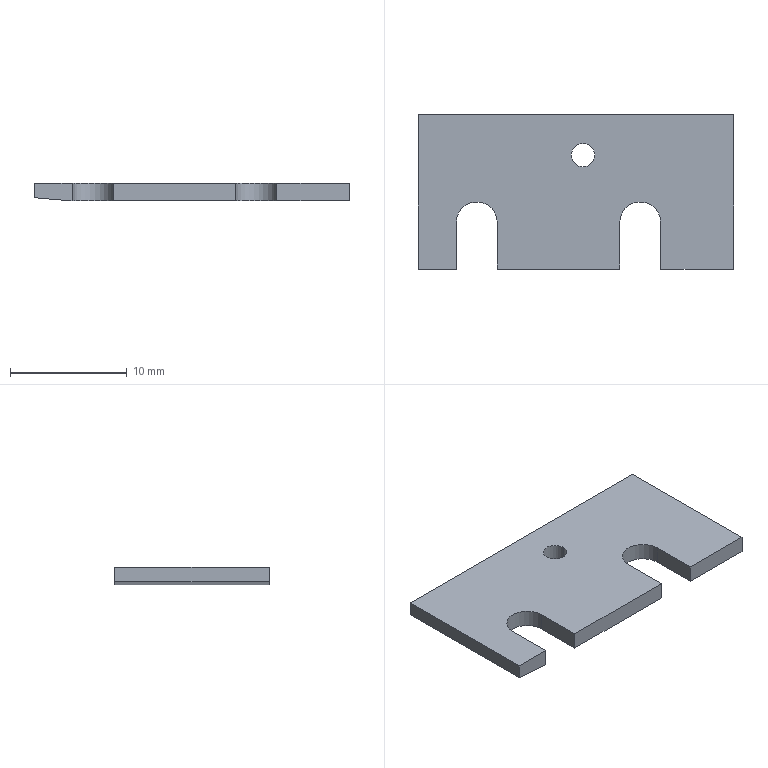Part | NX | 1 solid | 17 faces | box 27 x 13.2 x 1.5 mm | volume 468.259 mm3 | plane 13 | cylinder 4 | commonest cylinder face diameters 2 x2 3.5 x2
STEP:
#1=CARTESIAN_POINT('',(-113.5,7.2,-0.75));
#2=VERTEX_POINT('',#1);
#3=CARTESIAN_POINT('',(-113.5,-6.,-0.75));
#4=VERTEX_POINT('',#3);
#5=CARTESIAN_POINT('',(-113.5,0.,-0.75));
#6=DIRECTION('',(0.,-1.,0.));
#7=VECTOR('',#6,1000.);
#8=LINE('',#5,#7);
#9=EDGE_CURVE('',#2,#4,#8,.T.);
#10=ORIENTED_EDGE('',*,*,#9,.T.);
#11=CARTESIAN_POINT('',(-119.75,-6.,-0.75));
#12=VERTEX_POINT('',#11);
#13=CARTESIAN_POINT('',(0.,-6.,-0.75));
#14=DIRECTION('',(-1.,0.,0.));
#15=VECTOR('',#14,1000.);
#16=LINE('',#13,#15);
#17=EDGE_CURVE('',#4,#12,#16,.T.);
#18=ORIENTED_EDGE('',*,*,#17,.T.);
#19=CARTESIAN_POINT('',(-119.75,-2.,-0.75));
#20=VERTEX_POINT('',#19);
#21=CARTESIAN_POINT('',(-119.75,0.,-0.75));
#22=DIRECTION('',(0.,1.,0.));
#23=VECTOR('',#22,1000.);
#24=LINE('',#21,#23);
#25=EDGE_CURVE('',#12,#20,#24,.T.);
#26=ORIENTED_EDGE('',*,*,#25,.T.);
#27=CARTESIAN_POINT('',(-123.25,-2.,-0.75));
#28=VERTEX_POINT('',#27);
#29=CARTESIAN_POINT('',(-121.5,-2.,-0.75));
#30=DIRECTION('',(0.,0.,1.));
#31=DIRECTION('',(1.,0.,0.));
#32=AXIS2_PLACEMENT_3D('',#29,#30,#31);
#33=CIRCLE('',#32,1.75);
#34=EDGE_CURVE('',#20,#28,#33,.T.);
#35=ORIENTED_EDGE('',*,*,#34,.T.);
#36=CARTESIAN_POINT('',(-123.25,-6.,-0.75));
#37=VERTEX_POINT('',#36);
#38=CARTESIAN_POINT('',(-123.25,0.,-0.75));
#39=DIRECTION('',(0.,-1.,0.));
#40=VECTOR('',#39,1000.);
#41=LINE('',#38,#40);
#42=EDGE_CURVE('',#28,#37,#41,.T.);
#43=ORIENTED_EDGE('',*,*,#42,.T.);
#44=CARTESIAN_POINT('',(-133.75,-6.,-0.75));
#45=VERTEX_POINT('',#44);
#46=CARTESIAN_POINT('',(0.,-6.,-0.75));
#47=DIRECTION('',(-1.,0.,0.));
#48=VECTOR('',#47,1000.);
#49=LINE('',#46,#48);
#50=EDGE_CURVE('',#37,#45,#49,.T.);
#51=ORIENTED_EDGE('',*,*,#50,.T.);
#52=CARTESIAN_POINT('',(-133.75,-2.,-0.75));
#53=VERTEX_POINT('',#52);
#54=CARTESIAN_POINT('',(-133.75,0.,-0.75));
#55=DIRECTION('',(0.,1.,0.));
#56=VECTOR('',#55,1000.);
#57=LINE('',#54,#56);
#58=EDGE_CURVE('',#45,#53,#57,.T.);
#59=ORIENTED_EDGE('',*,*,#58,.T.);
#60=CARTESIAN_POINT('',(-137.25,-2.,-0.75));
#61=VERTEX_POINT('',#60);
#62=CARTESIAN_POINT('',(-135.5,-2.,-0.75));
#63=DIRECTION('',(0.,0.,1.));
#64=DIRECTION('',(1.,0.,0.));
#65=AXIS2_PLACEMENT_3D('',#62,#63,#64);
#66=CIRCLE('',#65,1.75);
#67=EDGE_CURVE('',#53,#61,#66,.T.);
#68=ORIENTED_EDGE('',*,*,#67,.T.);
#69=CARTESIAN_POINT('',(-137.25,-6.,-0.75));
#70=VERTEX_POINT('',#69);
#71=CARTESIAN_POINT('',(-137.25,0.,-0.75));
#72=DIRECTION('',(0.,-1.,0.));
#73=VECTOR('',#72,1000.);
#74=LINE('',#71,#73);
#75=EDGE_CURVE('',#61,#70,#74,.T.);
#76=ORIENTED_EDGE('',*,*,#75,.T.);
#77=CARTESIAN_POINT('',(-137.5,-6.,-0.75));
#78=VERTEX_POINT('',#77);
#79=CARTESIAN_POINT('',(0.,-6.,-0.75));
#80=DIRECTION('',(-1.,0.,0.));
#81=VECTOR('',#80,1000.);
#82=LINE('',#79,#81);
#83=EDGE_CURVE('',#70,#78,#82,.T.);
#84=ORIENTED_EDGE('',*,*,#83,.T.);
#85=CARTESIAN_POINT('',(-137.5,7.2,-0.75));
#86=VERTEX_POINT('',#85);
#87=CARTESIAN_POINT('',(-137.5,0.,-0.75));
#88=DIRECTION('',(0.,1.,0.));
#89=VECTOR('',#88,1000.);
#90=LINE('',#87,#89);
#91=EDGE_CURVE('',#78,#86,#90,.T.);
#92=ORIENTED_EDGE('',*,*,#91,.T.);
#93=CARTESIAN_POINT('',(0.,7.2,-0.75));
#94=DIRECTION('',(-1.,0.,0.));
#95=VECTOR('',#94,1000.);
#96=LINE('',#93,#95);
#97=EDGE_CURVE('',#2,#86,#96,.T.);
#98=ORIENTED_EDGE('',*,*,#97,.F.);
#99=EDGE_LOOP('',(#10,#18,#26,#35,#43,#51,#59,#68,#76,#84,#92,#98));
#100=FACE_BOUND('',#99,.T.);
#101=CARTESIAN_POINT('',(-127.4,3.75,-0.75));
#102=VERTEX_POINT('',#101);
#103=CARTESIAN_POINT('',(-125.4,3.75,-0.75));
#104=VERTEX_POINT('',#103);
#105=CARTESIAN_POINT('',(-126.4,3.75,-0.75));
#106=DIRECTION('',(0.,0.,-1.));
#107=DIRECTION('',(-1.,0.,0.));
#108=AXIS2_PLACEMENT_3D('',#105,#106,#107);
#109=CIRCLE('',#108,1.);
#110=EDGE_CURVE('',#102,#104,#109,.T.);
#111=ORIENTED_EDGE('',*,*,#110,.F.);
#112=CARTESIAN_POINT('',(-126.4,3.75,-0.75));
#113=DIRECTION('',(0.,0.,-1.));
#114=DIRECTION('',(-1.,0.,0.));
#115=AXIS2_PLACEMENT_3D('',#112,#113,#114);
#116=CIRCLE('',#115,1.);
#117=EDGE_CURVE('',#104,#102,#116,.T.);
#118=ORIENTED_EDGE('',*,*,#117,.F.);
#119=EDGE_LOOP('',(#111,#118));
#120=FACE_BOUND('',#119,.T.);
#121=CARTESIAN_POINT('',(-127.,0.,-0.75));
#122=DIRECTION('',(0.,0.,-1.));
#123=DIRECTION('',(0.,-1.,0.));
#124=AXIS2_PLACEMENT_3D('',#121,#122,#123);
#125=PLANE('',#124);
#126=ADVANCED_FACE('',(#100,#120),#125,.T.);
#127=ORIENTED_EDGE('',*,*,#9,.F.);
#128=CARTESIAN_POINT('',(-113.5,7.2,0.75));
#129=VERTEX_POINT('',#128);
#130=CARTESIAN_POINT('',(-113.5,7.2,0.));
#131=DIRECTION('',(0.,0.,1.));
#132=VECTOR('',#131,1000.);
#133=LINE('',#130,#132);
#134=EDGE_CURVE('',#2,#129,#133,.T.);
#135=ORIENTED_EDGE('',*,*,#134,.T.);
#136=CARTESIAN_POINT('',(-113.5,-6.,0.75));
#137=VERTEX_POINT('',#136);
#138=CARTESIAN_POINT('',(-113.5,0.,0.75));
#139=DIRECTION('',(0.,1.,0.));
#140=VECTOR('',#139,1000.);
#141=LINE('',#138,#140);
#142=EDGE_CURVE('',#137,#129,#141,.T.);
#143=ORIENTED_EDGE('',*,*,#142,.F.);
#144=CARTESIAN_POINT('',(-113.5,-6.,0.));
#145=DIRECTION('',(0.,0.,1.));
#146=VECTOR('',#145,1000.);
#147=LINE('',#144,#146);
#148=EDGE_CURVE('',#4,#137,#147,.T.);
#149=ORIENTED_EDGE('',*,*,#148,.F.);
#150=EDGE_LOOP('',(#127,#135,#143,#149));
#151=FACE_BOUND('',#150,.T.);
#152=CARTESIAN_POINT('',(-113.5,6.,-0.75));
#153=DIRECTION('',(-1.,0.,0.));
#154=DIRECTION('',(0.,0.,1.));
#155=AXIS2_PLACEMENT_3D('',#152,#153,#154);
#156=PLANE('',#155);
#157=ADVANCED_FACE('',(#151),#156,.F.);
#158=ORIENTED_EDGE('',*,*,#83,.F.);
#159=CARTESIAN_POINT('',(-137.25,-6.,0.75));
#160=VERTEX_POINT('',#159);
#161=CARTESIAN_POINT('',(-137.25,-6.,-0.9));
#162=DIRECTION('',(0.,0.,1.));
#163=VECTOR('',#162,1000.);
#164=LINE('',#161,#163);
#165=EDGE_CURVE('',#70,#160,#164,.T.);
#166=ORIENTED_EDGE('',*,*,#165,.T.);
#167=CARTESIAN_POINT('',(-140.5,-6.,0.75));
#168=VERTEX_POINT('',#167);
#169=CARTESIAN_POINT('',(0.,-6.,0.75));
#170=DIRECTION('',(-1.,0.,0.));
#171=VECTOR('',#170,1000.);
#172=LINE('',#169,#171);
#173=EDGE_CURVE('',#160,#168,#172,.T.);
#174=ORIENTED_EDGE('',*,*,#173,.T.);
#175=CARTESIAN_POINT('',(-140.5,-6.,-0.4875));
#176=VERTEX_POINT('',#175);
#177=CARTESIAN_POINT('',(-140.5,-6.,0.));
#178=DIRECTION('',(0.,0.,-1.));
#179=VECTOR('',#178,1000.);
#180=LINE('',#177,#179);
#181=EDGE_CURVE('',#168,#176,#180,.T.);
#182=ORIENTED_EDGE('',*,*,#181,.T.);
#183=CARTESIAN_POINT('',(0.,-6.,-12.78));
#184=DIRECTION('',(0.9962,0.,-0.08716));
#185=VECTOR('',#184,1000.);
#186=LINE('',#183,#185);
#187=EDGE_CURVE('',#176,#78,#186,.T.);
#188=ORIENTED_EDGE('',*,*,#187,.T.);
#189=EDGE_LOOP('',(#158,#166,#174,#182,#188));
#190=FACE_BOUND('',#189,.T.);
#191=CARTESIAN_POINT('',(-113.5,-6.,-0.75));
#192=DIRECTION('',(0.,1.,0.));
#193=DIRECTION('',(1.,0.,0.));
#194=AXIS2_PLACEMENT_3D('',#191,#192,#193);
#195=PLANE('',#194);
#196=ADVANCED_FACE('',(#190),#195,.F.);
#197=ORIENTED_EDGE('',*,*,#91,.F.);
#198=ORIENTED_EDGE('',*,*,#187,.F.);
#199=CARTESIAN_POINT('',(-140.5,7.2,-0.4875));
#200=VERTEX_POINT('',#199);
#201=CARTESIAN_POINT('',(-140.5,0.,-0.4875));
#202=DIRECTION('',(0.,1.,0.));
#203=VECTOR('',#202,1000.);
#204=LINE('',#201,#203);
#205=EDGE_CURVE('',#176,#200,#204,.T.);
#206=ORIENTED_EDGE('',*,*,#205,.T.);
#207=CARTESIAN_POINT('',(0.,7.2,-12.78));
#208=DIRECTION('',(0.9962,0.,-0.08716));
#209=VECTOR('',#208,1000.);
#210=LINE('',#207,#209);
#211=EDGE_CURVE('',#200,#86,#210,.T.);
#212=ORIENTED_EDGE('',*,*,#211,.T.);
#213=EDGE_LOOP('',(#197,#198,#206,#212));
#214=FACE_BOUND('',#213,.T.);
#215=CARTESIAN_POINT('',(-137.5,-6.,-0.75));
#216=DIRECTION('',(0.08716,0.,0.9962));
#217=DIRECTION('',(0.,-1.,0.));
#218=AXIS2_PLACEMENT_3D('',#215,#216,#217);
#219=PLANE('',#218);
#220=ADVANCED_FACE('',(#214),#219,.F.);
#221=ORIENTED_EDGE('',*,*,#97,.T.);
#222=ORIENTED_EDGE('',*,*,#211,.F.);
#223=CARTESIAN_POINT('',(-140.5,7.2,0.75));
#224=VERTEX_POINT('',#223);
#225=CARTESIAN_POINT('',(-140.5,7.2,0.));
#226=DIRECTION('',(0.,0.,-1.));
#227=VECTOR('',#226,1000.);
#228=LINE('',#225,#227);
#229=EDGE_CURVE('',#224,#200,#228,.T.);
#230=ORIENTED_EDGE('',*,*,#229,.F.);
#231=CARTESIAN_POINT('',(0.,7.2,0.75));
#232=DIRECTION('',(-1.,0.,0.));
#233=VECTOR('',#232,1000.);
#234=LINE('',#231,#233);
#235=EDGE_CURVE('',#129,#224,#234,.T.);
#236=ORIENTED_EDGE('',*,*,#235,.F.);
#237=ORIENTED_EDGE('',*,*,#134,.F.);
#238=EDGE_LOOP('',(#221,#222,#230,#236,#237));
#239=FACE_BOUND('',#238,.T.);
#240=CARTESIAN_POINT('',(-140.5,7.2,-0.75));
#241=DIRECTION('',(0.,-1.,0.));
#242=DIRECTION('',(0.,0.,-1.));
#243=AXIS2_PLACEMENT_3D('',#240,#241,#242);
#244=PLANE('',#243);
#245=ADVANCED_FACE('',(#239),#244,.F.);
#246=ORIENTED_EDGE('',*,*,#142,.T.);
#247=ORIENTED_EDGE('',*,*,#235,.T.);
#248=CARTESIAN_POINT('',(-140.5,0.,0.75));
#249=DIRECTION('',(0.,-1.,0.));
#250=VECTOR('',#249,1000.);
#251=LINE('',#248,#250);
#252=EDGE_CURVE('',#224,#168,#251,.T.);
#253=ORIENTED_EDGE('',*,*,#252,.T.);
#254=ORIENTED_EDGE('',*,*,#173,.F.);
#255=CARTESIAN_POINT('',(-137.25,-2.,0.75));
#256=VERTEX_POINT('',#255);
#257=CARTESIAN_POINT('',(-137.25,0.,0.75));
#258=DIRECTION('',(0.,-1.,0.));
#259=VECTOR('',#258,1000.);
#260=LINE('',#257,#259);
#261=EDGE_CURVE('',#256,#160,#260,.T.);
#262=ORIENTED_EDGE('',*,*,#261,.F.);
#263=CARTESIAN_POINT('',(-133.75,-2.,0.75));
#264=VERTEX_POINT('',#263);
#265=CARTESIAN_POINT('',(-135.5,-2.,0.75));
#266=DIRECTION('',(0.,0.,1.));
#267=DIRECTION('',(1.,0.,0.));
#268=AXIS2_PLACEMENT_3D('',#265,#266,#267);
#269=CIRCLE('',#268,1.75);
#270=EDGE_CURVE('',#264,#256,#269,.T.);
#271=ORIENTED_EDGE('',*,*,#270,.F.);
#272=CARTESIAN_POINT('',(-133.75,-6.,0.75));
#273=VERTEX_POINT('',#272);
#274=CARTESIAN_POINT('',(-133.75,0.,0.75));
#275=DIRECTION('',(0.,1.,0.));
#276=VECTOR('',#275,1000.);
#277=LINE('',#274,#276);
#278=EDGE_CURVE('',#273,#264,#277,.T.);
#279=ORIENTED_EDGE('',*,*,#278,.F.);
#280=CARTESIAN_POINT('',(-123.25,-6.,0.75));
#281=VERTEX_POINT('',#280);
#282=CARTESIAN_POINT('',(0.,-6.,0.75));
#283=DIRECTION('',(-1.,0.,0.));
#284=VECTOR('',#283,1000.);
#285=LINE('',#282,#284);
#286=EDGE_CURVE('',#281,#273,#285,.T.);
#287=ORIENTED_EDGE('',*,*,#286,.F.);
#288=CARTESIAN_POINT('',(-123.25,-2.,0.75));
#289=VERTEX_POINT('',#288);
#290=CARTESIAN_POINT('',(-123.25,0.,0.75));
#291=DIRECTION('',(0.,-1.,0.));
#292=VECTOR('',#291,1000.);
#293=LINE('',#290,#292);
#294=EDGE_CURVE('',#289,#281,#293,.T.);
#295=ORIENTED_EDGE('',*,*,#294,.F.);
#296=CARTESIAN_POINT('',(-119.75,-2.,0.75));
#297=VERTEX_POINT('',#296);
#298=CARTESIAN_POINT('',(-121.5,-2.,0.75));
#299=DIRECTION('',(0.,0.,1.));
#300=DIRECTION('',(1.,0.,0.));
#301=AXIS2_PLACEMENT_3D('',#298,#299,#300);
#302=CIRCLE('',#301,1.75);
#303=EDGE_CURVE('',#297,#289,#302,.T.);
#304=ORIENTED_EDGE('',*,*,#303,.F.);
#305=CARTESIAN_POINT('',(-119.75,-6.,0.75));
#306=VERTEX_POINT('',#305);
#307=CARTESIAN_POINT('',(-119.75,0.,0.75));
#308=DIRECTION('',(0.,1.,0.));
#309=VECTOR('',#308,1000.);
#310=LINE('',#307,#309);
#311=EDGE_CURVE('',#306,#297,#310,.T.);
#312=ORIENTED_EDGE('',*,*,#311,.F.);
#313=CARTESIAN_POINT('',(0.,-6.,0.75));
#314=DIRECTION('',(-1.,0.,0.));
#315=VECTOR('',#314,1000.);
#316=LINE('',#313,#315);
#317=EDGE_CURVE('',#137,#306,#316,.T.);
#318=ORIENTED_EDGE('',*,*,#317,.F.);
#319=EDGE_LOOP('',(#246,#247,#253,#254,#262,#271,#279,#287,#295,#304,#312,#318));
#320=FACE_BOUND('',#319,.T.);
#321=CARTESIAN_POINT('',(-127.4,3.75,0.75));
#322=VERTEX_POINT('',#321);
#323=CARTESIAN_POINT('',(-125.4,3.75,0.75));
#324=VERTEX_POINT('',#323);
#325=CARTESIAN_POINT('',(-126.4,3.75,0.75));
#326=DIRECTION('',(0.,0.,-1.));
#327=DIRECTION('',(-1.,0.,0.));
#328=AXIS2_PLACEMENT_3D('',#325,#326,#327);
#329=CIRCLE('',#328,1.);
#330=EDGE_CURVE('',#322,#324,#329,.T.);
#331=ORIENTED_EDGE('',*,*,#330,.T.);
#332=CARTESIAN_POINT('',(-126.4,3.75,0.75));
#333=DIRECTION('',(0.,0.,-1.));
#334=DIRECTION('',(-1.,0.,0.));
#335=AXIS2_PLACEMENT_3D('',#332,#333,#334);
#336=CIRCLE('',#335,1.);
#337=EDGE_CURVE('',#324,#322,#336,.T.);
#338=ORIENTED_EDGE('',*,*,#337,.T.);
#339=EDGE_LOOP('',(#331,#338));
#340=FACE_BOUND('',#339,.T.);
#341=CARTESIAN_POINT('',(-127.,0.,0.75));
#342=DIRECTION('',(0.,0.,-1.));
#343=DIRECTION('',(0.,-1.,0.));
#344=AXIS2_PLACEMENT_3D('',#341,#342,#343);
#345=PLANE('',#344);
#346=ADVANCED_FACE('',(#320,#340),#345,.F.);
#347=ORIENTED_EDGE('',*,*,#205,.F.);
#348=ORIENTED_EDGE('',*,*,#181,.F.);
#349=ORIENTED_EDGE('',*,*,#252,.F.);
#350=ORIENTED_EDGE('',*,*,#229,.T.);
#351=EDGE_LOOP('',(#347,#348,#349,#350));
#352=FACE_BOUND('',#351,.T.);
#353=CARTESIAN_POINT('',(-140.5,-6.,-0.75));
#354=DIRECTION('',(1.,0.,0.));
#355=DIRECTION('',(0.,1.,0.));
#356=AXIS2_PLACEMENT_3D('',#353,#354,#355);
#357=PLANE('',#356);
#358=ADVANCED_FACE('',(#352),#357,.F.);
#359=ORIENTED_EDGE('',*,*,#303,.T.);
#360=CARTESIAN_POINT('',(-123.25,-2.,0.75));
#361=DIRECTION('',(0.,0.,1.));
#362=VECTOR('',#361,1000.);
#363=LINE('',#360,#362);
#364=EDGE_CURVE('',#28,#289,#363,.T.);
#365=ORIENTED_EDGE('',*,*,#364,.F.);
#366=ORIENTED_EDGE('',*,*,#34,.F.);
#367=CARTESIAN_POINT('',(-119.75,-2.,0.75));
#368=DIRECTION('',(0.,0.,1.));
#369=VECTOR('',#368,1000.);
#370=LINE('',#367,#369);
#371=EDGE_CURVE('',#20,#297,#370,.T.);
#372=ORIENTED_EDGE('',*,*,#371,.T.);
#373=EDGE_LOOP('',(#359,#365,#366,#372));
#374=FACE_BOUND('',#373,.T.);
#375=CARTESIAN_POINT('',(-121.5,-2.,0.75));
#376=DIRECTION('',(0.,0.,1.));
#377=DIRECTION('',(1.,0.,0.));
#378=AXIS2_PLACEMENT_3D('',#375,#376,#377);
#379=CYLINDRICAL_SURFACE('',#378,1.75);
#380=ADVANCED_FACE('',(#374),#379,.F.);
#381=ORIENTED_EDGE('',*,*,#330,.F.);
#382=CARTESIAN_POINT('',(-127.4,3.75,0.75));
#383=DIRECTION('',(0.,0.,-1.));
#384=VECTOR('',#383,1000.);
#385=LINE('',#382,#384);
#386=EDGE_CURVE('',#102,#322,#385,.F.);
#387=ORIENTED_EDGE('',*,*,#386,.F.);
#388=ORIENTED_EDGE('',*,*,#110,.T.);
#389=CARTESIAN_POINT('',(-125.4,3.75,0.75));
#390=DIRECTION('',(0.,0.,-1.));
#391=VECTOR('',#390,1000.);
#392=LINE('',#389,#391);
#393=EDGE_CURVE('',#104,#324,#392,.F.);
#394=ORIENTED_EDGE('',*,*,#393,.T.);
#395=EDGE_LOOP('',(#381,#387,#388,#394));
#396=FACE_BOUND('',#395,.T.);
#397=CARTESIAN_POINT('',(-126.4,3.75,0.75));
#398=DIRECTION('',(0.,0.,-1.));
#399=DIRECTION('',(-1.,0.,0.));
#400=AXIS2_PLACEMENT_3D('',#397,#398,#399);
#401=CYLINDRICAL_SURFACE('',#400,1.);
#402=ADVANCED_FACE('',(#396),#401,.F.);
#403=CARTESIAN_POINT('',(-133.75,-2.,0.75));
#404=DIRECTION('',(0.,0.,1.));
#405=VECTOR('',#404,1000.);
#406=LINE('',#403,#405);
#407=EDGE_CURVE('',#53,#264,#406,.T.);
#408=ORIENTED_EDGE('',*,*,#407,.T.);
#409=ORIENTED_EDGE('',*,*,#270,.T.);
#410=CARTESIAN_POINT('',(-137.25,-2.,0.75));
#411=DIRECTION('',(0.,0.,1.));
#412=VECTOR('',#411,1000.);
#413=LINE('',#410,#412);
#414=EDGE_CURVE('',#61,#256,#413,.T.);
#415=ORIENTED_EDGE('',*,*,#414,.F.);
#416=ORIENTED_EDGE('',*,*,#67,.F.);
#417=EDGE_LOOP('',(#408,#409,#415,#416));
#418=FACE_BOUND('',#417,.T.);
#419=CARTESIAN_POINT('',(-135.5,-2.,0.75));
#420=DIRECTION('',(0.,0.,1.));
#421=DIRECTION('',(1.,0.,0.));
#422=AXIS2_PLACEMENT_3D('',#419,#420,#421);
#423=CYLINDRICAL_SURFACE('',#422,1.75);
#424=ADVANCED_FACE('',(#418),#423,.F.);
#425=CARTESIAN_POINT('',(-119.75,-6.,0.));
#426=DIRECTION('',(0.,0.,-1.));
#427=VECTOR('',#426,1000.);
#428=LINE('',#425,#427);
#429=EDGE_CURVE('',#306,#12,#428,.T.);
#430=ORIENTED_EDGE('',*,*,#429,.T.);
#431=ORIENTED_EDGE('',*,*,#17,.F.);
#432=ORIENTED_EDGE('',*,*,#148,.T.);
#433=ORIENTED_EDGE('',*,*,#317,.T.);
#434=EDGE_LOOP('',(#430,#431,#432,#433));
#435=FACE_BOUND('',#434,.T.);
#436=CARTESIAN_POINT('',(-113.5,-6.,-0.75));
#437=DIRECTION('',(0.,1.,0.));
#438=DIRECTION('',(1.,0.,0.));
#439=AXIS2_PLACEMENT_3D('',#436,#437,#438);
#440=PLANE('',#439);
#441=ADVANCED_FACE('',(#435),#440,.F.);
#442=CARTESIAN_POINT('',(-133.75,-6.,-0.9));
#443=DIRECTION('',(0.,0.,1.));
#444=VECTOR('',#443,1000.);
#445=LINE('',#442,#444);
#446=EDGE_CURVE('',#45,#273,#445,.T.);
#447=ORIENTED_EDGE('',*,*,#446,.F.);
#448=ORIENTED_EDGE('',*,*,#50,.F.);
#449=CARTESIAN_POINT('',(-123.25,-6.,0.));
#450=DIRECTION('',(0.,0.,1.));
#451=VECTOR('',#450,1000.);
#452=LINE('',#449,#451);
#453=EDGE_CURVE('',#37,#281,#452,.T.);
#454=ORIENTED_EDGE('',*,*,#453,.T.);
#455=ORIENTED_EDGE('',*,*,#286,.T.);
#456=EDGE_LOOP('',(#447,#448,#454,#455));
#457=FACE_BOUND('',#456,.T.);
#458=CARTESIAN_POINT('',(-113.5,-6.,-0.75));
#459=DIRECTION('',(0.,1.,0.));
#460=DIRECTION('',(1.,0.,0.));
#461=AXIS2_PLACEMENT_3D('',#458,#459,#460);
#462=PLANE('',#461);
#463=ADVANCED_FACE('',(#457),#462,.F.);
#464=ORIENTED_EDGE('',*,*,#42,.F.);
#465=ORIENTED_EDGE('',*,*,#364,.T.);
#466=ORIENTED_EDGE('',*,*,#294,.T.);
#467=ORIENTED_EDGE('',*,*,#453,.F.);
#468=EDGE_LOOP('',(#464,#465,#466,#467));
#469=FACE_BOUND('',#468,.T.);
#470=CARTESIAN_POINT('',(-123.25,-6.,-0.9));
#471=DIRECTION('',(-1.,0.,0.));
#472=DIRECTION('',(0.,0.,1.));
#473=AXIS2_PLACEMENT_3D('',#470,#471,#472);
#474=PLANE('',#473);
#475=ADVANCED_FACE('',(#469),#474,.F.);
#476=ORIENTED_EDGE('',*,*,#75,.F.);
#477=ORIENTED_EDGE('',*,*,#414,.T.);
#478=ORIENTED_EDGE('',*,*,#261,.T.);
#479=ORIENTED_EDGE('',*,*,#165,.F.);
#480=EDGE_LOOP('',(#476,#477,#478,#479));
#481=FACE_BOUND('',#480,.T.);
#482=CARTESIAN_POINT('',(-137.25,-6.,-0.9));
#483=DIRECTION('',(-1.,0.,0.));
#484=DIRECTION('',(0.,0.,1.));
#485=AXIS2_PLACEMENT_3D('',#482,#483,#484);
#486=PLANE('',#485);
#487=ADVANCED_FACE('',(#481),#486,.F.);
#488=ORIENTED_EDGE('',*,*,#25,.F.);
#489=ORIENTED_EDGE('',*,*,#429,.F.);
#490=ORIENTED_EDGE('',*,*,#311,.T.);
#491=ORIENTED_EDGE('',*,*,#371,.F.);
#492=EDGE_LOOP('',(#488,#489,#490,#491));
#493=FACE_BOUND('',#492,.T.);
#494=CARTESIAN_POINT('',(-119.75,-2.,-0.9));
#495=DIRECTION('',(1.,0.,0.));
#496=DIRECTION('',(0.,1.,0.));
#497=AXIS2_PLACEMENT_3D('',#494,#495,#496);
#498=PLANE('',#497);
#499=ADVANCED_FACE('',(#493),#498,.F.);
#500=ORIENTED_EDGE('',*,*,#278,.T.);
#501=ORIENTED_EDGE('',*,*,#407,.F.);
#502=ORIENTED_EDGE('',*,*,#58,.F.);
#503=ORIENTED_EDGE('',*,*,#446,.T.);
#504=EDGE_LOOP('',(#500,#501,#502,#503));
#505=FACE_BOUND('',#504,.T.);
#506=CARTESIAN_POINT('',(-133.75,-2.,-0.9));
#507=DIRECTION('',(1.,0.,0.));
#508=DIRECTION('',(0.,1.,0.));
#509=AXIS2_PLACEMENT_3D('',#506,#507,#508);
#510=PLANE('',#509);
#511=ADVANCED_FACE('',(#505),#510,.F.);
#512=ORIENTED_EDGE('',*,*,#386,.T.);
#513=ORIENTED_EDGE('',*,*,#337,.F.);
#514=ORIENTED_EDGE('',*,*,#393,.F.);
#515=ORIENTED_EDGE('',*,*,#117,.T.);
#516=EDGE_LOOP('',(#512,#513,#514,#515));
#517=FACE_BOUND('',#516,.T.);
#518=CARTESIAN_POINT('',(-126.4,3.75,0.75));
#519=DIRECTION('',(0.,0.,-1.));
#520=DIRECTION('',(-1.,0.,0.));
#521=AXIS2_PLACEMENT_3D('',#518,#519,#520);
#522=CYLINDRICAL_SURFACE('',#521,1.);
#523=ADVANCED_FACE('',(#517),#522,.F.);
#524=CLOSED_SHELL('',(#126,#157,#196,#220,#245,#346,#358,#380,#402,#424,#441,#463,#475,#487,#499,#511,#523));
#525=MANIFOLD_SOLID_BREP('',#524);
#526=(LENGTH_UNIT()NAMED_UNIT(*)SI_UNIT(.MILLI.,.METRE.));
#527=UNCERTAINTY_MEASURE_WITH_UNIT(LENGTH_MEASURE(0.00001),#526,'','');
#528=(NAMED_UNIT(*)PLANE_ANGLE_UNIT()SI_UNIT($,.RADIAN.));
#529=(NAMED_UNIT(*)SI_UNIT($,.STERADIAN.)SOLID_ANGLE_UNIT());
#530=(GEOMETRIC_REPRESENTATION_CONTEXT(3)GLOBAL_UNCERTAINTY_ASSIGNED_CONTEXT((#527))GLOBAL_UNIT_ASSIGNED_CONTEXT((#526,#528,#529))REPRESENTATION_CONTEXT('',''));
#531=ADVANCED_BREP_SHAPE_REPRESENTATION('',(#525),#530);